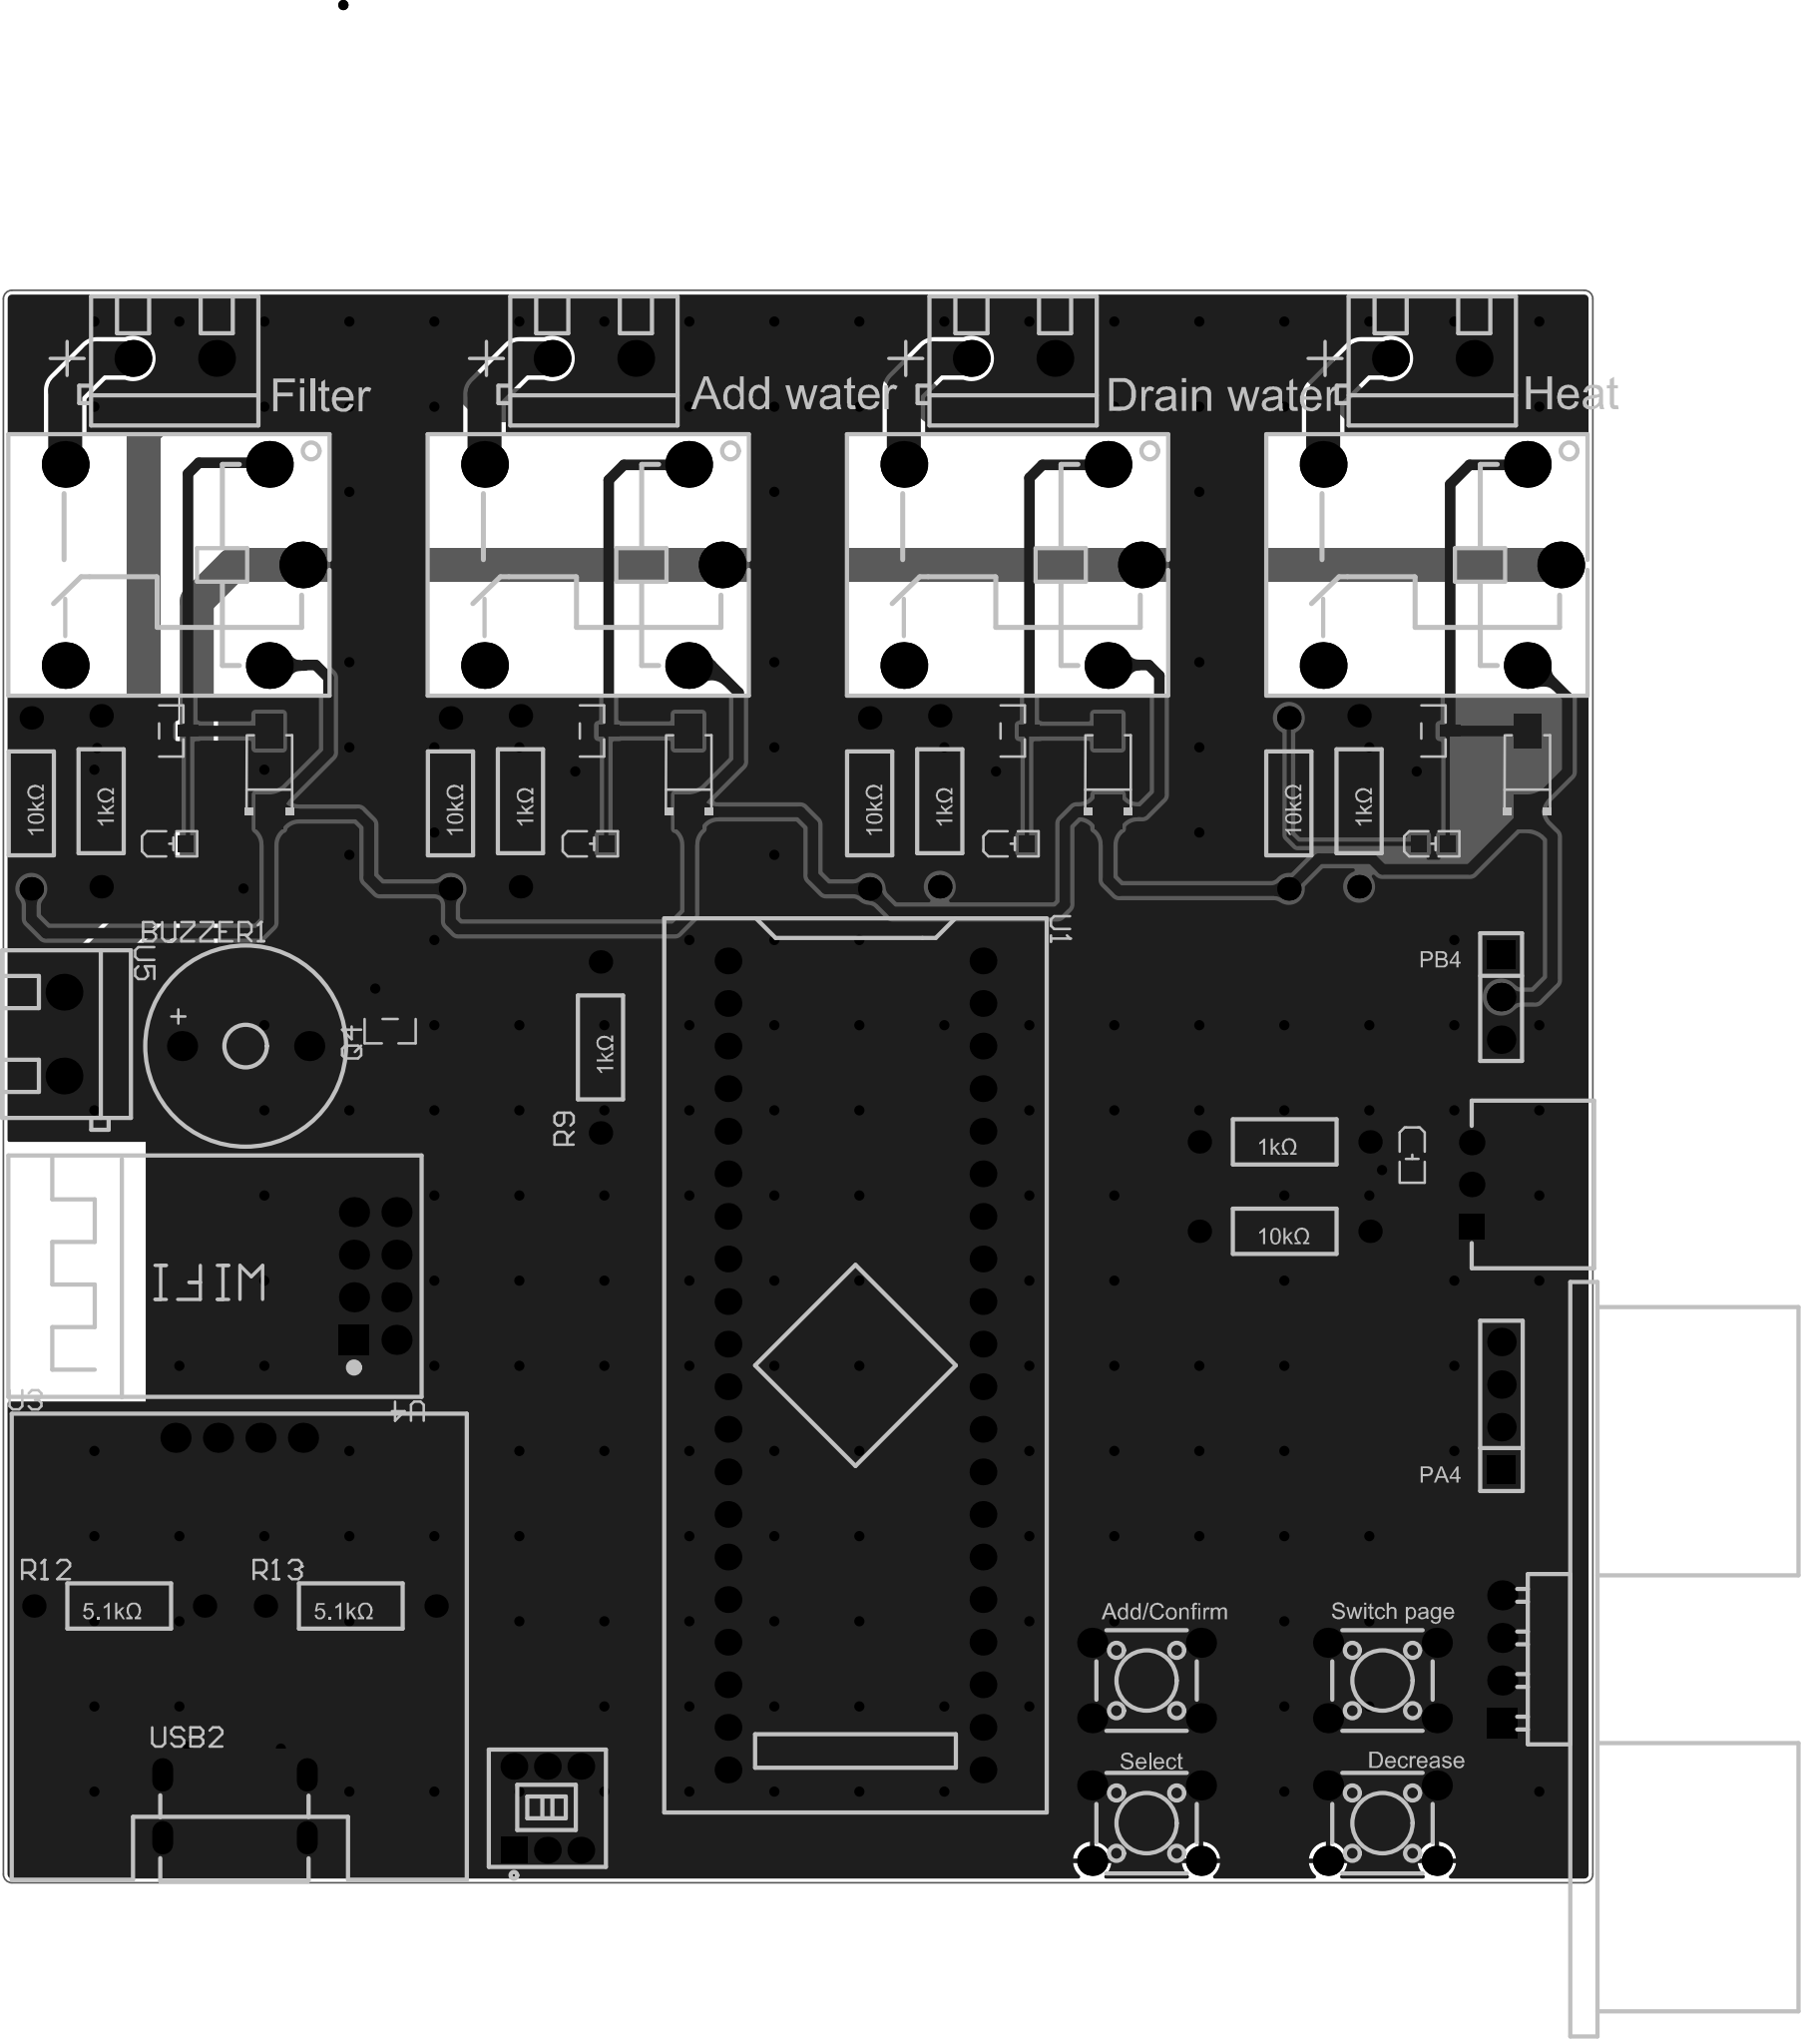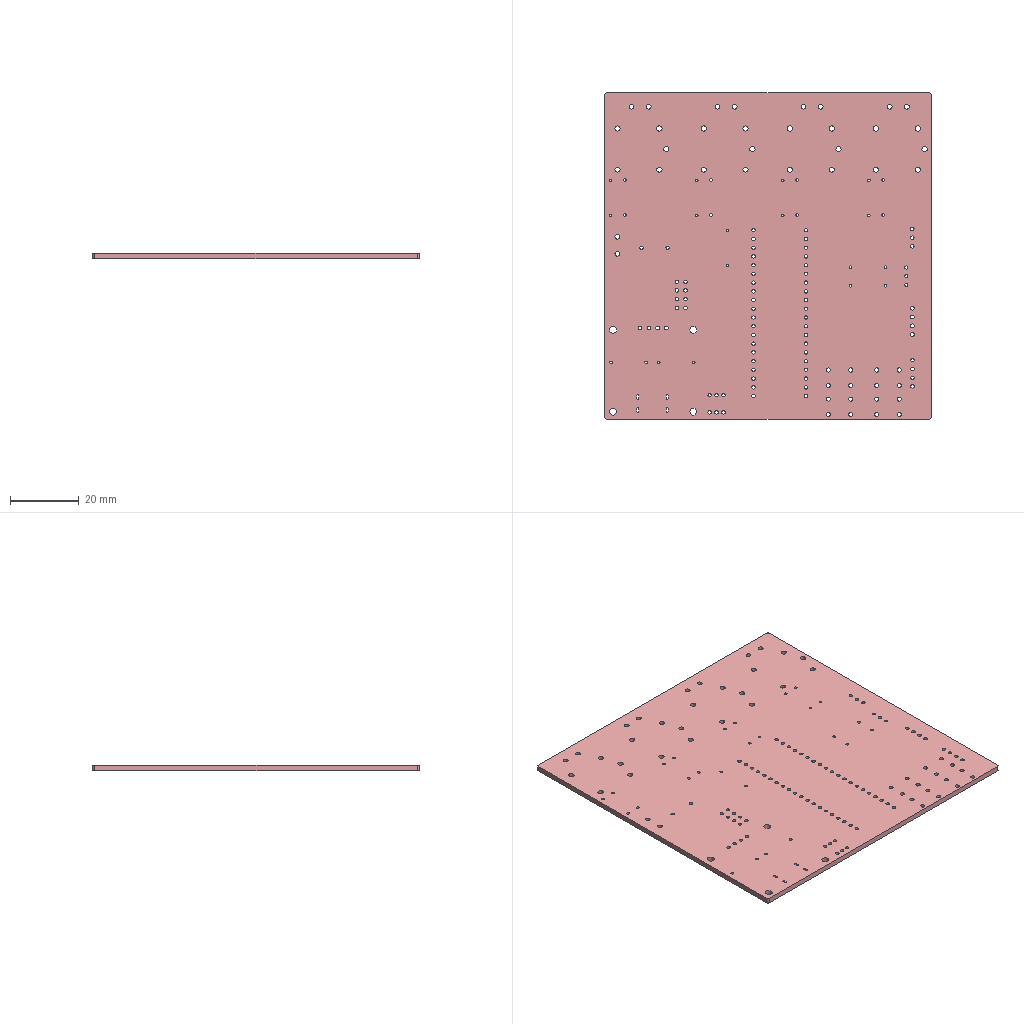Circuit board layout | Altium Designer | box 95 x 95 x 1.6 mm
Layer stack:
# Altium Designer layer stack of  (unit mm; dielectric type: 0 none, 1 core, 2 prepreg, 3 surface material)
index,name,kind,layer,copper_thickness_mm,dielectric_type,dielectric_thickness_mm,dielectric_material,dielectric_constant
0,Top Paste Mask Layer,other,,,,,,
1,Top Silkscreen Layer,other,,,,,,
2,Top Solder Mask Layer,dielectric,,,3,0.01,,3.3
3,Top Layer,copper,Top Layer,0.035,,,,
4,Dielectric1,dielectric,,,3,1.51,FR4,4.5
5,Bottom Layer,copper,Bottom Layer,0.035,,,,
6,Bottom Solder Mask Layer,dielectric,,,3,0.01,,3.3
7,Bottom Silkscreen Layer,other,,,,,,
8,Bottom Paste Mask Layer,other,,,,,,
# drill layer pairs: low layer,high layer
drill_pair,Top Layer,Bottom Layer
Part placement:
Designator,Comment,Layer,Footprint,Center-X(mm),Center-Y(mm),Rotation
BUZZER1,2.4kHz,TopLayer,BUZ-TH_BD12.0-P7.60-D0.6-FD,93.853,135.336,0
D1,1N4007A-AAF,TopLayer,SMA_L4.3-W2.6-LS5.0-RD,145.393,151.719,90
D2,1N4007A-AAF,TopLayer,SMA_L4.3-W2.6-LS5.0-RD,120.331,151.719,90
D3,1N4007A-AAF,TopLayer,SMA_L4.3-W2.6-LS5.0-RD,95.27,151.719,90
D4,1N4007A-AAF,TopLayer,SMA_L4.3-W2.6-LS5.0-RD,170.454,151.719,90
H2,PZ254V-11-03P,TopLayer,HDR-TH_3P-P2.54-V-M_PZ254V-11-03P,168.89,138.257,270
H3,PZ254V-11-04P,TopLayer,HDR-TH_4P-P2.54-V-M,168.91,113.873,90
Q1,SS8050,TopLayer,SOT-23-3_L2.9-W1.3-P1.90-LS2.4-BR,114.554,154.132,180
Q2,SS8050,TopLayer,SOT-23-3_L2.9-W1.3-P1.90-LS2.4-BR,139.7,154.132,180
Q3,SS8050,TopLayer,SOT-23-3_L2.9-W1.3-P1.90-LS2.4-BR,89.408,154.132,180
Q4,SS8050,TopLayer,SOT-23-3_L2.9-W1.3-P1.90-LS2.4-BR,102.489,136.225,90
Q5,SS8050,TopLayer,SOT-23-3_L2.9-W1.3-P1.90-LS2.4-BR,164.846,154.132,180
R1,10kΩ,TopLayer,RES-TH_BD2.7-L6.2-P10.20-D0.4,106.096,149.814,270
R2,10kΩ,TopLayer,RES-TH_BD2.7-L6.2-P10.20-D0.4,131.15,149.814,270
R3,10kΩ,TopLayer,RES-TH_BD2.7-L6.2-P10.20-D0.4,81.043,149.814,270
R4,10kΩ,TopLayer,RES-TH_BD2.7-L6.2-P10.20-D0.4,156.203,149.814,270
R5,1kΩ,TopLayer,RES-TH_BD2.7-L6.2-P10.20-D0.4,135.34,149.941,90
R6,1kΩ,TopLayer,RES-TH_BD2.7-L6.2-P10.20-D0.4,110.278,149.941,90
R7,1kΩ,TopLayer,RES-TH_BD2.7-L6.2-P10.20-D0.4,85.217,149.941,90
R8,1kΩ,TopLayer,RES-TH_BD2.7-L6.2-P10.20-D0.4,160.401,149.941,90
R9,1kΩ,TopLayer,RES-TH_BD2.7-L6.2-P10.20-D0.4,115.062,135.256,90
R10,10kΩ,TopLayer,RES-TH_BD2.7-L6.2-P10.20-D0.4,155.956,124.287,180
R11,1kΩ,TopLayer,RES-TH_BD2.7-L6.2-P10.20-D0.4,155.956,129.621,180
R12,5.1kΩ,TopLayer,RES-TH_BD2.7-L6.2-P10.20-D0.4,86.298,101.935,0
R13,5.1kΩ,TopLayer,RES-TH_BD2.7-L6.2-P10.20-D0.4,100.138,101.935,0
RLY2,SRD-05VDC-SL-C,TopLayer,RELAY-TH_SRD-XXVDC-XL-C,115.231,164.038,180
RLY3,SRD-05VDC-SL-C,TopLayer,RELAY-TH_SRD-XXVDC-XL-C,140.293,164.038,180
RLY4,SRD-05VDC-SL-C,TopLayer,RELAY-TH_SRD-XXVDC-XL-C,90.17,164.038,180
RLY5,SRD-05VDC-SL-C,TopLayer,RELAY-TH_SRD-XXVDC-XL-C,165.354,164.038,180
SW1,TS665CJ,TopLayer,SW-TH_4P-L6.0-W6.0-P4.50-LS6.5,161.798,97.49,0
SW2,TS665CJ,TopLayer,SW-TH_4P-L6.0-W6.0-P4.50-LS6.5,147.701,97.49,0
SW3,TS665CJ,TopLayer,SW-TH_4P-L6.0-W6.0-P4.50-LS6.5,161.798,88.981,0
SW4,TS665CJ,TopLayer,SW-TH_4P-L6.0-W6.0-P4.50-LS6.5,147.701,88.981,0
SW5,TK-6700-1,TopLayer,SW-TH_TK-6700-1,111.887,89.87,0
U1,LCKFB-DKX-STM32F103C8T6,TopLayer,CONN-TH_L53.3-W22.9_STM32F103C8T6-CARD,130.302,116.286,270
U2,HC-SR04,TopLayer,TH_HC-SR04V,168.96,98.76,90
U3,HS96L03W2C03,TopLayer,OLED-TH_L27.8-W27.2-P2.54_C9900033791,93.472,111.968,0
U4,2.4GHz,TopLayer,WIFIM-TH_8P-L24.7-W14.4-P2.54,101.6,121.62,180
U8,KF301-5.0-2P,TopLayer,CONN-TH_P5.00_KF301-5.0-2P,114.669,176.357,180
U9,KF301-5.0-2P,TopLayer,CONN-TH_P5.00_KF301-5.0-2P,139.722,176.357,180
U10,KF301-5.0-2P,TopLayer,CONN-TH_P5.00_KF301-5.0-2P,89.616,176.357,180
U13,KF301-5.0-2P,TopLayer,CONN-TH_P5.00_KF301-5.0-2P,164.776,176.357,180
U14,WAFER-XH2.54-3PWZ,TopLayer,CONN-TH_3P-P2.50_WAFER-XH2.54-3PWZ,167.132,127.081,90
USB2,,TopLayer,USB__TYPE-C-6P,93.218,90.251,0
LED1,GL0603UR01,TopLayer,LED0603-FD,114.554,147.401,180
LED2,GL0603UR01,TopLayer,LED0603-FD,139.7,147.401,180
LED3,GL0603UR01,TopLayer,LED0603-FD,89.408,147.401,180
LED4,GL0603UR01,TopLayer,LED0603-FD,164.846,147.401,180
LED5,GL0603UR01,TopLayer,LED0603-FD,163.576,128.732,90
U5,KF301-5.0-2P,TopLayer,CONN-TH_P5.00_KF301-5.0-2P,82.998,136.05,270
Pad and via stacks:
# Altium Designer via and pad stacks of  (unit mm). Each distinct definition once, with the count of objects using it.
# via: kind,start_layer,end_layer,hole_mm,diameter_mm,mode(0 simple;1 top-mid-bottom;2 full stack),diameter_per_layer,count,example_net
# pad: kind,layer,hole_mm,hole_type(0 round;1 square;2 slot),plating,top_size,top_shape(1 round;2 rect;3 octagon;9 rounded rect),mid_size,bottom_size,mode,footprint,size_per_layer,count,example
pad,Multi-Layer,1,0,plated,1.8x1.8,1,1.8x1.8,1.8x1.8,0,BUZ-TH_BD12.0-P7.60-D0.6-FD,,2,BUZZER1.2
pad,Multi-Layer,1.02,0,plated,1.7x1.7,2,1.7x1.7,1.7x1.7,0,HDR-TH_3P-P2.54-V-M_PZ254V-11-03P,,1,H2.1
pad,Multi-Layer,1.02,0,plated,1.7x1.7,1,1.7x1.7,1.7x1.7,0,HDR-TH_3P-P2.54-V-M_PZ254V-11-03P,,2,H2.2
pad,Multi-Layer,1.1,0,plated,1.7x1.7,2,1.7x1.7,1.7x1.7,0,HDR-TH_4P-P2.54-V-M,,1,H3.1
pad,Multi-Layer,1.1,0,plated,1.7x1.7,1,1.7x1.7,1.7x1.7,0,HDR-TH_4P-P2.54-V-M,,3,H3.2
pad,Multi-Layer,0.8,0,plated,1.4x1.4,1,1.4x1.4,1.4x1.4,0,RES-TH_BD2.7-L6.2-P10.20-D0.4,,26,R1.1
pad,Multi-Layer,1.524,0,plated,2.794x2.794,1,2.794x2.794,2.794x2.794,0,RELAY-TH_SRD-XXVDC-XL-C,,20,RLY2.2
pad,Multi-Layer,1.2,0,plated,1.8x1.8,1,1.8x1.8,1.8x1.8,0,SW-TH_4P-L6.0-W6.0-P4.50-LS6.5,,16,SW1.1
pad,Multi-Layer,1,0,plated,1.6x1.6,2,1.6x1.6,1.6x1.6,0,SW-TH_TK-6700-1,,1,SW5.1
pad,Multi-Layer,1,0,plated,1.6x1.6,1,1.6x1.6,1.6x1.6,0,SW-TH_TK-6700-1,,5,SW5.2
pad,Multi-Layer,1,0,plated,1.6x1.6,1,1.6x1.6,1.6x1.6,0,CONN-TH_L53.3-W22.9_STM32F103C8T6-CARD,,40,U1.1
pad,Multi-Layer,1.001,0,plated,1.8x1.8,1,1.8x1.8,1.8x1.8,0,TH_HC-SR04V,,3,U2.4
pad,Multi-Layer,1.001,0,plated,1.8x1.8,2,1.8x1.8,1.8x1.8,0,TH_HC-SR04V,,1,U2.1
pad,Multi-Layer,1.05,0,plated,1.8x1.8,1,1.8x1.8,1.8x1.8,0,OLED-TH_L27.8-W27.2-P2.54_C9900033791,,4,U3.1
pad,Multi-Layer,1,0,plated,1.8x1.8,1,1.8x1.8,1.8x1.8,0,WIFIM-TH_8P-L24.7-W14.4-P2.54,,7,U4.8
pad,Multi-Layer,1,0,plated,1.8x1.8,2,1.8x1.8,1.8x1.8,0,WIFIM-TH_8P-L24.7-W14.4-P2.54,,1,U4.1
pad,Multi-Layer,1.4,0,plated,2.2x2.2,1,2.2x2.2,2.2x2.2,0,CONN-TH_P5.00_KF301-5.0-2P,,10,U8.1
pad,Multi-Layer,0.9144,0,plated,1.524x1.524,2,1.524x1.524,1.524x1.524,0,CONN-TH_3P-P2.50_WAFER-XH2.54-3PWZ,,1,U14.1
pad,Multi-Layer,0.9144,0,plated,1.524x1.524,1,1.524x1.524,1.524x1.524,0,CONN-TH_3P-P2.50_WAFER-XH2.54-3PWZ,,2,U14.2
pad,Multi-Layer,0.6,2,plated,1.25x2,1,1.25x2,1.25x2,0,USB_ TYPE-C-6P,,4,USB2.8
pad,Top Layer,0,0,plated,2.046x1.62,2,2.046x1.62,2.046x1.62,0,SMA_L4.3-W2.6-LS5.0-RD,,8,D1.2
pad,Top Layer,0,0,plated,1.25x0.7,2,1.25x0.7,1.25x0.7,0,SOT-23-3_L2.9-W1.3-P1.90-LS2.4-BR,,15,Q1.1
pad,Top Layer,0,0,plated,0.7x2.032,2,0.7x2.032,0.7x2.032,0,USB_ TYPE-C-6P,,2,USB2.A5
pad,Top Layer,0,0,plated,0.8x2.032,2,0.8x2.032,0.8x2.032,0,USB_ TYPE-C-6P,,2,USB2.B9
pad,Top Layer,0,0,plated,0.9x2.032,2,0.9x2.032,0.9x2.032,0,USB_ TYPE-C-6P,,2,USB2.B12
pad,Top Layer,0,0,plated,1x0.8999,2,1x0.8999,1x0.8999,0,LED0603-FD,,10,LED1.1
via,Top Layer,Bottom Layer,0.3048,0.61,0,,190,GND
Copper pours:
name,layer,net,type(0 solid;1 hatched;2 none)
Top Layer-GND,Top Layer,GND,0
Bottom Layer-GND,Bottom Layer,GND,0